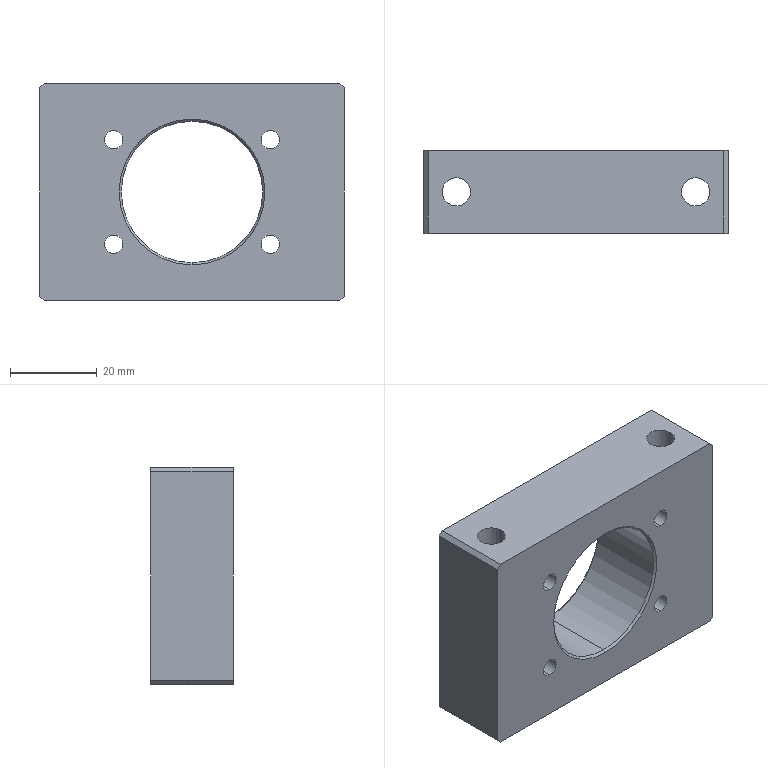Part | STEP file | Sliding plate 2 | 1 solid | 34 faces | box 70 x 19 x 50 mm | volume 40709 mm3 | cylinder 18 | plane 12 | cone 4 | commonest cylinder face diameters 4.2 x8 6.5 x4 12 x4 32.5 x2